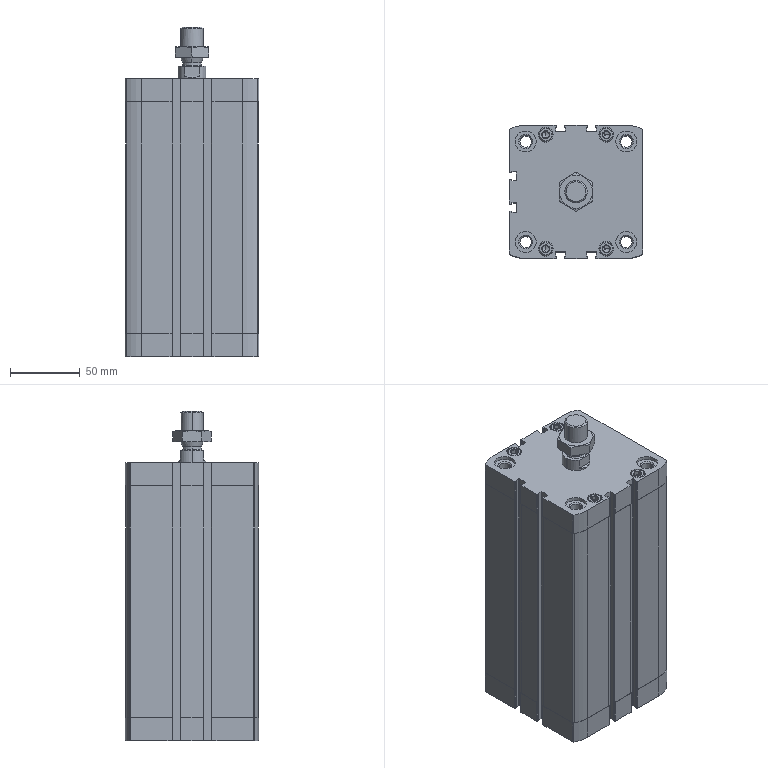Part | SolidWorks | features AEMSimFeature 1 | 3 solids | 507 faces | box 95.5 x 95.5 x 235.9 mm | volume 1025771 mm3 | plane 235 | cylinder 188 | cone 80 | spline 4 | commonest cylinder face diameters 0.8 x48 0.4 x24 8.376 x16 10 x16 10.7 x16 15 x16